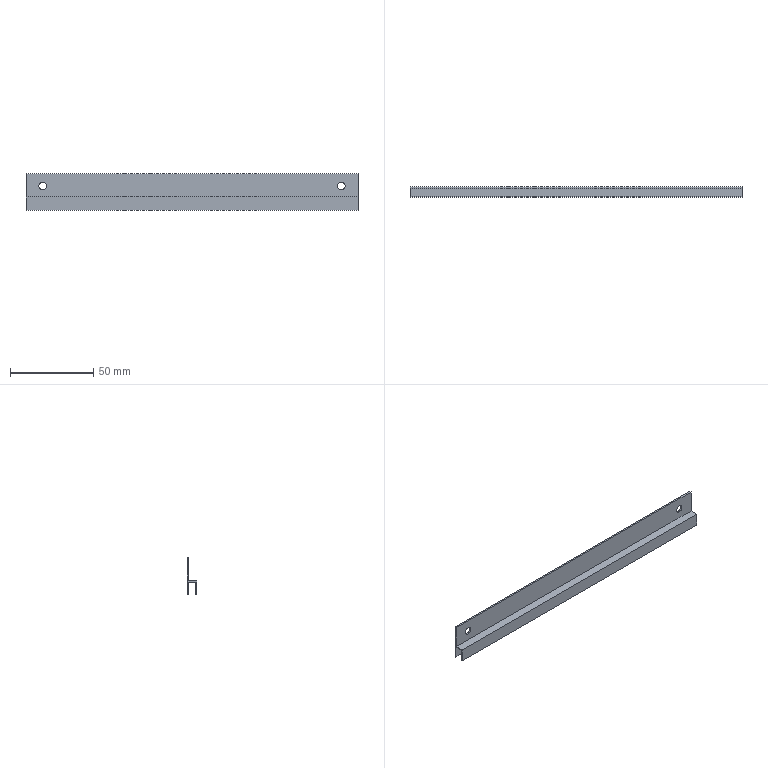Part | NX | features solid 2 | 1 solid | 16 faces | box 200 x 6 x 22 mm | volume 5843 mm3 | plane 12 | cylinder 4 | commonest cylinder face diameters 4.5 x4
STEP:
#1=CARTESIAN_POINT('',(-55.,2180.05,-879.75));
#2=VERTEX_POINT('',#1);
#3=CARTESIAN_POINT('',(-55.,2180.05,-887.));
#4=VERTEX_POINT('',#3);
#5=CARTESIAN_POINT('',(-55.,2180.05,-879.75));
#6=DIRECTION('',(0.,0.,-1.));
#7=VECTOR('',#6,1000.);
#8=LINE('',#5,#7);
#9=EDGE_CURVE('',#2,#4,#8,.T.);
#10=ORIENTED_EDGE('',*,*,#9,.T.);
#11=CARTESIAN_POINT('',(-255.,2180.05,-887.));
#12=VERTEX_POINT('',#11);
#13=CARTESIAN_POINT('',(-55.,2180.05,-887.));
#14=DIRECTION('',(-1.,0.,0.));
#15=VECTOR('',#14,1000.);
#16=LINE('',#13,#15);
#17=EDGE_CURVE('',#4,#12,#16,.T.);
#18=ORIENTED_EDGE('',*,*,#17,.T.);
#19=CARTESIAN_POINT('',(-255.,2180.05,-879.75));
#20=VERTEX_POINT('',#19);
#21=CARTESIAN_POINT('',(-255.,2180.05,-887.));
#22=DIRECTION('',(0.,0.,1.));
#23=VECTOR('',#22,1000.);
#24=LINE('',#21,#23);
#25=EDGE_CURVE('',#12,#20,#24,.T.);
#26=ORIENTED_EDGE('',*,*,#25,.T.);
#27=CARTESIAN_POINT('',(-255.,2180.05,-879.75));
#28=DIRECTION('',(1.,0.,0.));
#29=VECTOR('',#28,1000.);
#30=LINE('',#27,#29);
#31=EDGE_CURVE('',#20,#2,#30,.T.);
#32=ORIENTED_EDGE('',*,*,#31,.T.);
#33=EDGE_LOOP('',(#10,#18,#26,#32));
#34=FACE_BOUND('',#33,.T.);
#35=CARTESIAN_POINT('',(-55.,2180.05,-880.));
#36=DIRECTION('',(0.,1.,0.));
#37=DIRECTION('',(0.,0.,1.));
#38=AXIS2_PLACEMENT_3D('',#35,#36,#37);
#39=PLANE('',#38);
#40=ADVANCED_FACE('',(#34),#39,.T.);
#41=CARTESIAN_POINT('',(-55.,2184.55,-879.75));
#42=VERTEX_POINT('',#41);
#43=CARTESIAN_POINT('',(-55.,2184.55,-879.75));
#44=DIRECTION('',(0.,-1.,0.));
#45=VECTOR('',#44,1000.);
#46=LINE('',#43,#45);
#47=EDGE_CURVE('',#42,#2,#46,.T.);
#48=ORIENTED_EDGE('',*,*,#47,.T.);
#49=ORIENTED_EDGE('',*,*,#31,.F.);
#50=CARTESIAN_POINT('',(-255.,2184.55,-879.75));
#51=VERTEX_POINT('',#50);
#52=CARTESIAN_POINT('',(-255.,2180.05,-879.75));
#53=DIRECTION('',(0.,1.,0.));
#54=VECTOR('',#53,1000.);
#55=LINE('',#52,#54);
#56=EDGE_CURVE('',#20,#51,#55,.T.);
#57=ORIENTED_EDGE('',*,*,#56,.T.);
#58=CARTESIAN_POINT('',(-255.,2184.55,-879.75));
#59=DIRECTION('',(1.,0.,0.));
#60=VECTOR('',#59,1000.);
#61=LINE('',#58,#60);
#62=EDGE_CURVE('',#51,#42,#61,.T.);
#63=ORIENTED_EDGE('',*,*,#62,.T.);
#64=EDGE_LOOP('',(#48,#49,#57,#63));
#65=FACE_BOUND('',#64,.T.);
#66=CARTESIAN_POINT('',(-55.,2185.8,-879.75));
#67=DIRECTION('',(0.,0.,-1.));
#68=DIRECTION('',(0.,1.,0.));
#69=AXIS2_PLACEMENT_3D('',#66,#67,#68);
#70=PLANE('',#69);
#71=ADVANCED_FACE('',(#65),#70,.T.);
#72=CARTESIAN_POINT('',(-55.,2184.55,-887.));
#73=VERTEX_POINT('',#72);
#74=CARTESIAN_POINT('',(-55.,2184.55,-887.));
#75=DIRECTION('',(0.,0.,1.));
#76=VECTOR('',#75,1000.);
#77=LINE('',#74,#76);
#78=EDGE_CURVE('',#73,#42,#77,.T.);
#79=ORIENTED_EDGE('',*,*,#78,.T.);
#80=ORIENTED_EDGE('',*,*,#62,.F.);
#81=CARTESIAN_POINT('',(-255.,2184.55,-887.));
#82=VERTEX_POINT('',#81);
#83=CARTESIAN_POINT('',(-255.,2184.55,-879.75));
#84=DIRECTION('',(0.,0.,-1.));
#85=VECTOR('',#84,1000.);
#86=LINE('',#83,#85);
#87=EDGE_CURVE('',#51,#82,#86,.T.);
#88=ORIENTED_EDGE('',*,*,#87,.T.);
#89=CARTESIAN_POINT('',(-255.,2184.55,-887.));
#90=DIRECTION('',(1.,0.,0.));
#91=VECTOR('',#90,1000.);
#92=LINE('',#89,#91);
#93=EDGE_CURVE('',#82,#73,#92,.T.);
#94=ORIENTED_EDGE('',*,*,#93,.T.);
#95=EDGE_LOOP('',(#79,#80,#88,#94));
#96=FACE_BOUND('',#95,.T.);
#97=CARTESIAN_POINT('',(-55.,2184.55,-887.));
#98=DIRECTION('',(0.,-1.,0.));
#99=DIRECTION('',(0.,0.,-1.));
#100=AXIS2_PLACEMENT_3D('',#97,#98,#99);
#101=PLANE('',#100);
#102=ADVANCED_FACE('',(#96),#101,.T.);
#103=CARTESIAN_POINT('',(-55.,2185.3,-887.));
#104=VERTEX_POINT('',#103);
#105=CARTESIAN_POINT('',(-55.,2184.55,-887.));
#106=DIRECTION('',(0.,1.,0.));
#107=VECTOR('',#106,1000.);
#108=LINE('',#105,#107);
#109=EDGE_CURVE('',#73,#104,#108,.T.);
#110=ORIENTED_EDGE('',*,*,#109,.F.);
#111=ORIENTED_EDGE('',*,*,#93,.F.);
#112=CARTESIAN_POINT('',(-255.,2185.3,-887.));
#113=VERTEX_POINT('',#112);
#114=CARTESIAN_POINT('',(-255.,2184.55,-887.));
#115=DIRECTION('',(0.,1.,0.));
#116=VECTOR('',#115,1000.);
#117=LINE('',#114,#116);
#118=EDGE_CURVE('',#82,#113,#117,.T.);
#119=ORIENTED_EDGE('',*,*,#118,.T.);
#120=CARTESIAN_POINT('',(-255.,2185.3,-887.));
#121=DIRECTION('',(1.,0.,0.));
#122=VECTOR('',#121,1000.);
#123=LINE('',#120,#122);
#124=EDGE_CURVE('',#113,#104,#123,.T.);
#125=ORIENTED_EDGE('',*,*,#124,.T.);
#126=EDGE_LOOP('',(#110,#111,#119,#125));
#127=FACE_BOUND('',#126,.T.);
#128=CARTESIAN_POINT('',(-55.,2184.55,-887.));
#129=DIRECTION('',(0.,0.,1.));
#130=DIRECTION('',(1.,0.,0.));
#131=AXIS2_PLACEMENT_3D('',#128,#129,#130);
#132=PLANE('',#131);
#133=ADVANCED_FACE('',(#127),#132,.F.);
#134=CARTESIAN_POINT('',(-55.,2185.3,-865.));
#135=VERTEX_POINT('',#134);
#136=CARTESIAN_POINT('',(-55.,2185.3,-887.));
#137=DIRECTION('',(0.,0.,1.));
#138=VECTOR('',#137,1000.);
#139=LINE('',#136,#138);
#140=EDGE_CURVE('',#104,#135,#139,.T.);
#141=ORIENTED_EDGE('',*,*,#140,.F.);
#142=ORIENTED_EDGE('',*,*,#124,.F.);
#143=CARTESIAN_POINT('',(-255.,2185.3,-865.));
#144=VERTEX_POINT('',#143);
#145=CARTESIAN_POINT('',(-255.,2185.3,-887.));
#146=DIRECTION('',(0.,0.,1.));
#147=VECTOR('',#146,1000.);
#148=LINE('',#145,#147);
#149=EDGE_CURVE('',#113,#144,#148,.T.);
#150=ORIENTED_EDGE('',*,*,#149,.T.);
#151=CARTESIAN_POINT('',(-255.,2185.3,-865.));
#152=DIRECTION('',(1.,0.,0.));
#153=VECTOR('',#152,1000.);
#154=LINE('',#151,#153);
#155=EDGE_CURVE('',#144,#135,#154,.T.);
#156=ORIENTED_EDGE('',*,*,#155,.T.);
#157=EDGE_LOOP('',(#141,#142,#150,#156));
#158=FACE_BOUND('',#157,.T.);
#159=CARTESIAN_POINT('',(-65.,2185.3,-874.65));
#160=VERTEX_POINT('',#159);
#161=CARTESIAN_POINT('',(-65.,2185.3,-870.15));
#162=VERTEX_POINT('',#161);
#163=CARTESIAN_POINT('',(-65.,2185.3,-872.4));
#164=DIRECTION('',(0.,1.,0.));
#165=DIRECTION('',(0.,0.,-1.));
#166=AXIS2_PLACEMENT_3D('',#163,#164,#165);
#167=CIRCLE('',#166,2.25);
#168=EDGE_CURVE('',#160,#162,#167,.T.);
#169=ORIENTED_EDGE('',*,*,#168,.F.);
#170=CARTESIAN_POINT('',(-65.,2185.3,-872.4));
#171=DIRECTION('',(0.,1.,0.));
#172=DIRECTION('',(0.,0.,1.));
#173=AXIS2_PLACEMENT_3D('',#170,#171,#172);
#174=CIRCLE('',#173,2.25);
#175=EDGE_CURVE('',#162,#160,#174,.T.);
#176=ORIENTED_EDGE('',*,*,#175,.F.);
#177=EDGE_LOOP('',(#169,#176));
#178=FACE_BOUND('',#177,.T.);
#179=CARTESIAN_POINT('',(-245.,2185.3,-870.15));
#180=VERTEX_POINT('',#179);
#181=CARTESIAN_POINT('',(-245.,2185.3,-874.65));
#182=VERTEX_POINT('',#181);
#183=CARTESIAN_POINT('',(-245.,2185.3,-872.4));
#184=DIRECTION('',(0.,1.,0.));
#185=DIRECTION('',(0.,0.,1.));
#186=AXIS2_PLACEMENT_3D('',#183,#184,#185);
#187=CIRCLE('',#186,2.25);
#188=EDGE_CURVE('',#180,#182,#187,.T.);
#189=ORIENTED_EDGE('',*,*,#188,.F.);
#190=CARTESIAN_POINT('',(-245.,2185.3,-872.4));
#191=DIRECTION('',(0.,1.,0.));
#192=DIRECTION('',(0.,0.,-1.));
#193=AXIS2_PLACEMENT_3D('',#190,#191,#192);
#194=CIRCLE('',#193,2.25);
#195=EDGE_CURVE('',#182,#180,#194,.T.);
#196=ORIENTED_EDGE('',*,*,#195,.F.);
#197=EDGE_LOOP('',(#189,#196));
#198=FACE_BOUND('',#197,.T.);
#199=CARTESIAN_POINT('',(-55.,2185.3,-887.));
#200=DIRECTION('',(0.,-1.,0.));
#201=DIRECTION('',(0.,0.,-1.));
#202=AXIS2_PLACEMENT_3D('',#199,#200,#201);
#203=PLANE('',#202);
#204=ADVANCED_FACE('',(#158,#178,#198),#203,.F.);
#205=CARTESIAN_POINT('',(-55.,2184.3,-865.));
#206=VERTEX_POINT('',#205);
#207=CARTESIAN_POINT('',(-55.,2184.3,-865.));
#208=DIRECTION('',(0.,1.,0.));
#209=VECTOR('',#208,1000.);
#210=LINE('',#207,#209);
#211=EDGE_CURVE('',#206,#135,#210,.T.);
#212=ORIENTED_EDGE('',*,*,#211,.T.);
#213=ORIENTED_EDGE('',*,*,#155,.F.);
#214=CARTESIAN_POINT('',(-255.,2184.3,-865.));
#215=VERTEX_POINT('',#214);
#216=CARTESIAN_POINT('',(-255.,2185.3,-865.));
#217=DIRECTION('',(0.,-1.,0.));
#218=VECTOR('',#217,1000.);
#219=LINE('',#216,#218);
#220=EDGE_CURVE('',#144,#215,#219,.T.);
#221=ORIENTED_EDGE('',*,*,#220,.T.);
#222=CARTESIAN_POINT('',(-255.,2184.3,-865.));
#223=DIRECTION('',(1.,0.,0.));
#224=VECTOR('',#223,1000.);
#225=LINE('',#222,#224);
#226=EDGE_CURVE('',#215,#206,#225,.T.);
#227=ORIENTED_EDGE('',*,*,#226,.T.);
#228=EDGE_LOOP('',(#212,#213,#221,#227));
#229=FACE_BOUND('',#228,.T.);
#230=CARTESIAN_POINT('',(-130.,2182.3,-865.));
#231=DIRECTION('',(0.,0.,1.));
#232=DIRECTION('',(0.,-1.,0.));
#233=AXIS2_PLACEMENT_3D('',#230,#231,#232);
#234=PLANE('',#233);
#235=ADVANCED_FACE('',(#229),#234,.T.);
#236=CARTESIAN_POINT('',(-55.,2184.3,-879.));
#237=VERTEX_POINT('',#236);
#238=CARTESIAN_POINT('',(-55.,2184.3,-865.));
#239=DIRECTION('',(0.,0.,-1.));
#240=VECTOR('',#239,1000.);
#241=LINE('',#238,#240);
#242=EDGE_CURVE('',#206,#237,#241,.T.);
#243=ORIENTED_EDGE('',*,*,#242,.F.);
#244=ORIENTED_EDGE('',*,*,#226,.F.);
#245=CARTESIAN_POINT('',(-255.,2184.3,-879.));
#246=VERTEX_POINT('',#245);
#247=CARTESIAN_POINT('',(-255.,2184.3,-865.));
#248=DIRECTION('',(0.,0.,-1.));
#249=VECTOR('',#248,1000.);
#250=LINE('',#247,#249);
#251=EDGE_CURVE('',#215,#246,#250,.T.);
#252=ORIENTED_EDGE('',*,*,#251,.T.);
#253=CARTESIAN_POINT('',(-255.,2184.3,-879.));
#254=DIRECTION('',(1.,0.,0.));
#255=VECTOR('',#254,1000.);
#256=LINE('',#253,#255);
#257=EDGE_CURVE('',#246,#237,#256,.T.);
#258=ORIENTED_EDGE('',*,*,#257,.T.);
#259=EDGE_LOOP('',(#243,#244,#252,#258));
#260=FACE_BOUND('',#259,.T.);
#261=CARTESIAN_POINT('',(-65.,2184.3,-874.65));
#262=VERTEX_POINT('',#261);
#263=CARTESIAN_POINT('',(-65.,2184.3,-870.15));
#264=VERTEX_POINT('',#263);
#265=CARTESIAN_POINT('',(-65.,2184.3,-872.4));
#266=DIRECTION('',(0.,-1.,0.));
#267=DIRECTION('',(0.,0.,-1.));
#268=AXIS2_PLACEMENT_3D('',#265,#266,#267);
#269=CIRCLE('',#268,2.25);
#270=EDGE_CURVE('',#262,#264,#269,.T.);
#271=ORIENTED_EDGE('',*,*,#270,.F.);
#272=CARTESIAN_POINT('',(-65.,2184.3,-872.4));
#273=DIRECTION('',(0.,-1.,0.));
#274=DIRECTION('',(0.,0.,1.));
#275=AXIS2_PLACEMENT_3D('',#272,#273,#274);
#276=CIRCLE('',#275,2.25);
#277=EDGE_CURVE('',#264,#262,#276,.T.);
#278=ORIENTED_EDGE('',*,*,#277,.F.);
#279=EDGE_LOOP('',(#271,#278));
#280=FACE_BOUND('',#279,.T.);
#281=CARTESIAN_POINT('',(-245.,2184.3,-874.65));
#282=VERTEX_POINT('',#281);
#283=CARTESIAN_POINT('',(-245.,2184.3,-870.15));
#284=VERTEX_POINT('',#283);
#285=CARTESIAN_POINT('',(-245.,2184.3,-872.4));
#286=DIRECTION('',(0.,-1.,0.));
#287=DIRECTION('',(0.,0.,-1.));
#288=AXIS2_PLACEMENT_3D('',#285,#286,#287);
#289=CIRCLE('',#288,2.25);
#290=EDGE_CURVE('',#282,#284,#289,.T.);
#291=ORIENTED_EDGE('',*,*,#290,.F.);
#292=CARTESIAN_POINT('',(-245.,2184.3,-872.4));
#293=DIRECTION('',(0.,-1.,0.));
#294=DIRECTION('',(0.,0.,1.));
#295=AXIS2_PLACEMENT_3D('',#292,#293,#294);
#296=CIRCLE('',#295,2.25);
#297=EDGE_CURVE('',#284,#282,#296,.T.);
#298=ORIENTED_EDGE('',*,*,#297,.F.);
#299=EDGE_LOOP('',(#291,#298));
#300=FACE_BOUND('',#299,.T.);
#301=CARTESIAN_POINT('',(-55.,2184.3,-865.));
#302=DIRECTION('',(0.,1.,0.));
#303=DIRECTION('',(0.,0.,1.));
#304=AXIS2_PLACEMENT_3D('',#301,#302,#303);
#305=PLANE('',#304);
#306=ADVANCED_FACE('',(#260,#280,#300),#305,.F.);
#307=CARTESIAN_POINT('',(-55.,2179.3,-879.));
#308=VERTEX_POINT('',#307);
#309=CARTESIAN_POINT('',(-55.,2184.3,-879.));
#310=DIRECTION('',(0.,-1.,0.));
#311=VECTOR('',#310,1000.);
#312=LINE('',#309,#311);
#313=EDGE_CURVE('',#237,#308,#312,.T.);
#314=ORIENTED_EDGE('',*,*,#313,.F.);
#315=ORIENTED_EDGE('',*,*,#257,.F.);
#316=CARTESIAN_POINT('',(-255.,2179.3,-879.));
#317=VERTEX_POINT('',#316);
#318=CARTESIAN_POINT('',(-255.,2184.3,-879.));
#319=DIRECTION('',(0.,-1.,0.));
#320=VECTOR('',#319,1000.);
#321=LINE('',#318,#320);
#322=EDGE_CURVE('',#246,#317,#321,.T.);
#323=ORIENTED_EDGE('',*,*,#322,.T.);
#324=CARTESIAN_POINT('',(-255.,2179.3,-879.));
#325=DIRECTION('',(1.,0.,0.));
#326=VECTOR('',#325,1000.);
#327=LINE('',#324,#326);
#328=EDGE_CURVE('',#317,#308,#327,.T.);
#329=ORIENTED_EDGE('',*,*,#328,.T.);
#330=EDGE_LOOP('',(#314,#315,#323,#329));
#331=FACE_BOUND('',#330,.T.);
#332=CARTESIAN_POINT('',(-55.,2185.8,-879.));
#333=DIRECTION('',(0.,0.,-1.));
#334=DIRECTION('',(0.,1.,0.));
#335=AXIS2_PLACEMENT_3D('',#332,#333,#334);
#336=PLANE('',#335);
#337=ADVANCED_FACE('',(#331),#336,.F.);
#338=CARTESIAN_POINT('',(-55.,2179.3,-887.));
#339=VERTEX_POINT('',#338);
#340=CARTESIAN_POINT('',(-55.,2179.3,-879.));
#341=DIRECTION('',(0.,0.,-1.));
#342=VECTOR('',#341,1000.);
#343=LINE('',#340,#342);
#344=EDGE_CURVE('',#308,#339,#343,.T.);
#345=ORIENTED_EDGE('',*,*,#344,.F.);
#346=ORIENTED_EDGE('',*,*,#328,.F.);
#347=CARTESIAN_POINT('',(-255.,2179.3,-887.));
#348=VERTEX_POINT('',#347);
#349=CARTESIAN_POINT('',(-255.,2179.3,-879.));
#350=DIRECTION('',(0.,0.,-1.));
#351=VECTOR('',#350,1000.);
#352=LINE('',#349,#351);
#353=EDGE_CURVE('',#317,#348,#352,.T.);
#354=ORIENTED_EDGE('',*,*,#353,.T.);
#355=CARTESIAN_POINT('',(-255.,2179.3,-887.));
#356=DIRECTION('',(1.,0.,0.));
#357=VECTOR('',#356,1000.);
#358=LINE('',#355,#357);
#359=EDGE_CURVE('',#348,#339,#358,.T.);
#360=ORIENTED_EDGE('',*,*,#359,.T.);
#361=EDGE_LOOP('',(#345,#346,#354,#360));
#362=FACE_BOUND('',#361,.T.);
#363=CARTESIAN_POINT('',(-55.,2179.3,-880.));
#364=DIRECTION('',(0.,1.,0.));
#365=DIRECTION('',(0.,0.,1.));
#366=AXIS2_PLACEMENT_3D('',#363,#364,#365);
#367=PLANE('',#366);
#368=ADVANCED_FACE('',(#362),#367,.F.);
#369=CARTESIAN_POINT('',(-55.,2179.3,-887.));
#370=DIRECTION('',(0.,1.,0.));
#371=VECTOR('',#370,1000.);
#372=LINE('',#369,#371);
#373=EDGE_CURVE('',#339,#4,#372,.T.);
#374=ORIENTED_EDGE('',*,*,#373,.F.);
#375=ORIENTED_EDGE('',*,*,#359,.F.);
#376=CARTESIAN_POINT('',(-255.,2179.3,-887.));
#377=DIRECTION('',(0.,1.,0.));
#378=VECTOR('',#377,1000.);
#379=LINE('',#376,#378);
#380=EDGE_CURVE('',#348,#12,#379,.T.);
#381=ORIENTED_EDGE('',*,*,#380,.T.);
#382=ORIENTED_EDGE('',*,*,#17,.F.);
#383=EDGE_LOOP('',(#374,#375,#381,#382));
#384=FACE_BOUND('',#383,.T.);
#385=CARTESIAN_POINT('',(-55.,2178.8,-887.));
#386=DIRECTION('',(0.,0.,1.));
#387=DIRECTION('',(1.,0.,0.));
#388=AXIS2_PLACEMENT_3D('',#385,#386,#387);
#389=PLANE('',#388);
#390=ADVANCED_FACE('',(#384),#389,.F.);
#391=ORIENTED_EDGE('',*,*,#353,.F.);
#392=ORIENTED_EDGE('',*,*,#322,.F.);
#393=ORIENTED_EDGE('',*,*,#251,.F.);
#394=ORIENTED_EDGE('',*,*,#220,.F.);
#395=ORIENTED_EDGE('',*,*,#149,.F.);
#396=ORIENTED_EDGE('',*,*,#118,.F.);
#397=ORIENTED_EDGE('',*,*,#87,.F.);
#398=ORIENTED_EDGE('',*,*,#56,.F.);
#399=ORIENTED_EDGE('',*,*,#25,.F.);
#400=ORIENTED_EDGE('',*,*,#380,.F.);
#401=EDGE_LOOP('',(#391,#392,#393,#394,#395,#396,#397,#398,#399,#400));
#402=FACE_BOUND('',#401,.T.);
#403=CARTESIAN_POINT('',(-255.,2182.3,-880.));
#404=DIRECTION('',(-1.,0.,0.));
#405=DIRECTION('',(0.,1.,0.));
#406=AXIS2_PLACEMENT_3D('',#403,#404,#405);
#407=PLANE('',#406);
#408=ADVANCED_FACE('',(#402),#407,.T.);
#409=ORIENTED_EDGE('',*,*,#47,.F.);
#410=ORIENTED_EDGE('',*,*,#78,.F.);
#411=ORIENTED_EDGE('',*,*,#109,.T.);
#412=ORIENTED_EDGE('',*,*,#140,.T.);
#413=ORIENTED_EDGE('',*,*,#211,.F.);
#414=ORIENTED_EDGE('',*,*,#242,.T.);
#415=ORIENTED_EDGE('',*,*,#313,.T.);
#416=ORIENTED_EDGE('',*,*,#344,.T.);
#417=ORIENTED_EDGE('',*,*,#373,.T.);
#418=ORIENTED_EDGE('',*,*,#9,.F.);
#419=EDGE_LOOP('',(#409,#410,#411,#412,#413,#414,#415,#416,#417,#418));
#420=FACE_BOUND('',#419,.T.);
#421=CARTESIAN_POINT('',(-55.,2182.3,-880.));
#422=DIRECTION('',(1.,0.,0.));
#423=DIRECTION('',(0.,-1.,0.));
#424=AXIS2_PLACEMENT_3D('',#421,#422,#423);
#425=PLANE('',#424);
#426=ADVANCED_FACE('',(#420),#425,.T.);
#427=ORIENTED_EDGE('',*,*,#168,.T.);
#428=CARTESIAN_POINT('',(-65.,2185.3,-870.15));
#429=DIRECTION('',(0.,-1.,0.));
#430=VECTOR('',#429,1000.);
#431=LINE('',#428,#430);
#432=EDGE_CURVE('',#162,#264,#431,.T.);
#433=ORIENTED_EDGE('',*,*,#432,.T.);
#434=ORIENTED_EDGE('',*,*,#277,.T.);
#435=CARTESIAN_POINT('',(-65.,2185.3,-874.65));
#436=DIRECTION('',(0.,-1.,0.));
#437=VECTOR('',#436,1000.);
#438=LINE('',#435,#437);
#439=EDGE_CURVE('',#262,#160,#438,.F.);
#440=ORIENTED_EDGE('',*,*,#439,.T.);
#441=EDGE_LOOP('',(#427,#433,#434,#440));
#442=FACE_BOUND('',#441,.T.);
#443=CARTESIAN_POINT('',(-65.,2185.801,-872.4));
#444=DIRECTION('',(0.,-1.,0.));
#445=DIRECTION('',(0.,0.,-1.));
#446=AXIS2_PLACEMENT_3D('',#443,#444,#445);
#447=CYLINDRICAL_SURFACE('',#446,2.25);
#448=ADVANCED_FACE('',(#442),#447,.F.);
#449=ORIENTED_EDGE('',*,*,#439,.F.);
#450=ORIENTED_EDGE('',*,*,#270,.T.);
#451=ORIENTED_EDGE('',*,*,#432,.F.);
#452=ORIENTED_EDGE('',*,*,#175,.T.);
#453=EDGE_LOOP('',(#449,#450,#451,#452));
#454=FACE_BOUND('',#453,.T.);
#455=CARTESIAN_POINT('',(-65.,2185.801,-872.4));
#456=DIRECTION('',(0.,-1.,0.));
#457=DIRECTION('',(0.,0.,-1.));
#458=AXIS2_PLACEMENT_3D('',#455,#456,#457);
#459=CYLINDRICAL_SURFACE('',#458,2.25);
#460=ADVANCED_FACE('',(#454),#459,.F.);
#461=CARTESIAN_POINT('',(-245.,2184.3,-874.65));
#462=DIRECTION('',(0.,1.,0.));
#463=VECTOR('',#462,1000.);
#464=LINE('',#461,#463);
#465=EDGE_CURVE('',#282,#182,#464,.T.);
#466=ORIENTED_EDGE('',*,*,#465,.T.);
#467=ORIENTED_EDGE('',*,*,#195,.T.);
#468=CARTESIAN_POINT('',(-245.,2184.3,-870.15));
#469=DIRECTION('',(0.,1.,0.));
#470=VECTOR('',#469,1000.);
#471=LINE('',#468,#470);
#472=EDGE_CURVE('',#180,#284,#471,.F.);
#473=ORIENTED_EDGE('',*,*,#472,.T.);
#474=ORIENTED_EDGE('',*,*,#297,.T.);
#475=EDGE_LOOP('',(#466,#467,#473,#474));
#476=FACE_BOUND('',#475,.T.);
#477=CARTESIAN_POINT('',(-245.,2185.8,-872.4));
#478=DIRECTION('',(0.,1.,0.));
#479=DIRECTION('',(0.,0.,1.));
#480=AXIS2_PLACEMENT_3D('',#477,#478,#479);
#481=CYLINDRICAL_SURFACE('',#480,2.25);
#482=ADVANCED_FACE('',(#476),#481,.F.);
#483=ORIENTED_EDGE('',*,*,#472,.F.);
#484=ORIENTED_EDGE('',*,*,#188,.T.);
#485=ORIENTED_EDGE('',*,*,#465,.F.);
#486=ORIENTED_EDGE('',*,*,#290,.T.);
#487=EDGE_LOOP('',(#483,#484,#485,#486));
#488=FACE_BOUND('',#487,.T.);
#489=CARTESIAN_POINT('',(-245.,2185.8,-872.4));
#490=DIRECTION('',(0.,1.,0.));
#491=DIRECTION('',(0.,0.,1.));
#492=AXIS2_PLACEMENT_3D('',#489,#490,#491);
#493=CYLINDRICAL_SURFACE('',#492,2.25);
#494=ADVANCED_FACE('',(#488),#493,.F.);
#495=CLOSED_SHELL('',(#40,#71,#102,#133,#204,#235,#306,#337,#368,#390,#408,#426,#448,#460,#482,#494));
#496=MANIFOLD_SOLID_BREP('',#495);
#497=(LENGTH_UNIT()NAMED_UNIT(*)SI_UNIT(.MILLI.,.METRE.));
#498=UNCERTAINTY_MEASURE_WITH_UNIT(LENGTH_MEASURE(0.00001),#497,'','');
#499=(NAMED_UNIT(*)PLANE_ANGLE_UNIT()SI_UNIT($,.RADIAN.));
#500=(NAMED_UNIT(*)SI_UNIT($,.STERADIAN.)SOLID_ANGLE_UNIT());
#501=(GEOMETRIC_REPRESENTATION_CONTEXT(3)GLOBAL_UNCERTAINTY_ASSIGNED_CONTEXT((#498))GLOBAL_UNIT_ASSIGNED_CONTEXT((#497,#499,#500))REPRESENTATION_CONTEXT('',''));
#502=ADVANCED_BREP_SHAPE_REPRESENTATION('',(#496),#501);